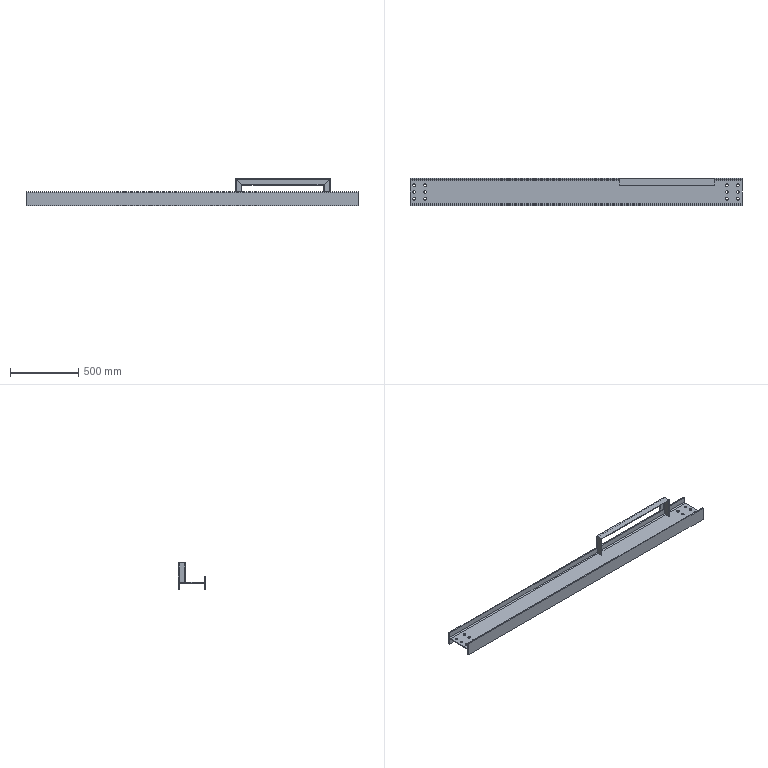Part | STEP file | 休息台主梁1主体_Default<As Machined> | 4 solids | 81 faces | box 2430 x 200 x 200 mm | volume 6806772 mm3 | plane 44 | cylinder 37 | commonest cylinder face diameters 19 x24 2.66 x6 16 x4 11 x3